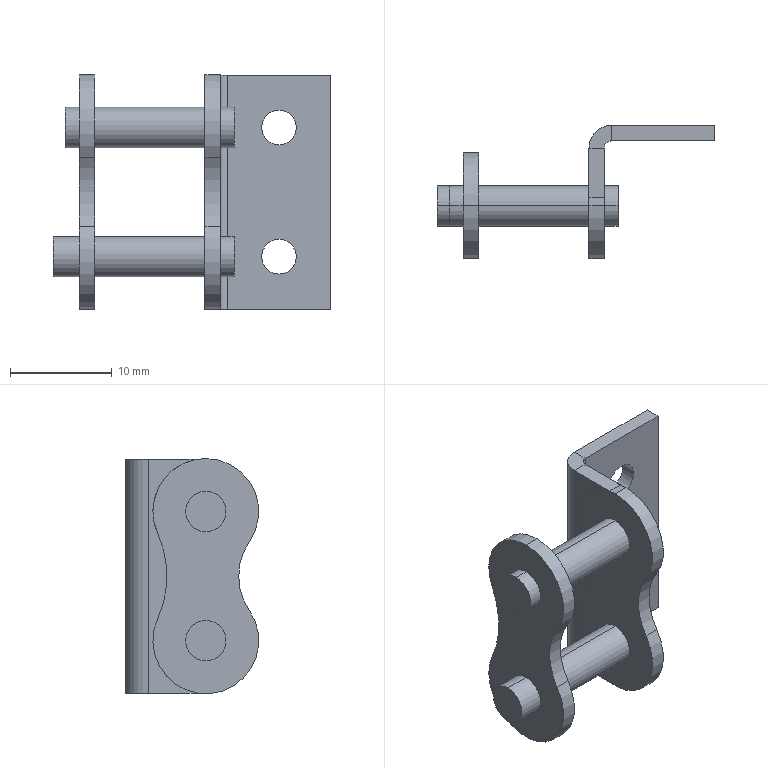Part | SolidWorks | features MoveFace 9, 3DProfileFeature 1, BaseBody 1, EdgeFlange 1, FlatPattern 1, HoleWzd 1, SMBaseFlange 1, SheetMetal 1 | 2 solids | 50 faces | box 27.296 x 13.105 x 23.11 mm | volume 1387 mm3 | cylinder 31 | plane 19 | commonest cylinder face diameters 3.98 x12 10.41 x8 3.4 x4 20 x3 12 x2 1.473 x1
STEP:
#1=CARTESIAN_POINT('',(12.2,6.4,-11.));
#2=VERTEX_POINT('',#1);
#3=CARTESIAN_POINT('',(12.2,6.4,-14.4));
#4=VERTEX_POINT('',#3);
#5=CARTESIAN_POINT('',(12.2,6.4,-12.7));
#6=DIRECTION('',(0.,-1.,0.));
#7=DIRECTION('',(1.,0.,0.));
#8=AXIS2_PLACEMENT_3D('',#5,#6,#7);
#9=CIRCLE('',#8,1.7);
#10=EDGE_CURVE('',#2,#4,#9,.T.);
#11=ORIENTED_EDGE('',*,*,#10,.T.);
#12=CARTESIAN_POINT('',(12.2,7.9,-14.4));
#13=VERTEX_POINT('',#12);
#14=CARTESIAN_POINT('',(12.2,7.9,-14.4));
#15=DIRECTION('',(0.,1.,0.));
#16=VECTOR('',#15,1000.);
#17=LINE('',#14,#16);
#18=EDGE_CURVE('',#4,#13,#17,.T.);
#19=ORIENTED_EDGE('',*,*,#18,.T.);
#20=CARTESIAN_POINT('',(12.2,7.9,-11.));
#21=VERTEX_POINT('',#20);
#22=CARTESIAN_POINT('',(12.2,7.9,-12.7));
#23=DIRECTION('',(0.,1.,0.));
#24=DIRECTION('',(0.,0.,1.));
#25=AXIS2_PLACEMENT_3D('',#22,#23,#24);
#26=CIRCLE('',#25,1.7);
#27=EDGE_CURVE('',#13,#21,#26,.T.);
#28=ORIENTED_EDGE('',*,*,#27,.T.);
#29=CARTESIAN_POINT('',(12.2,7.9,-11.));
#30=DIRECTION('',(0.,1.,0.));
#31=VECTOR('',#30,1000.);
#32=LINE('',#29,#31);
#33=EDGE_CURVE('',#2,#21,#32,.T.);
#34=ORIENTED_EDGE('',*,*,#33,.F.);
#35=EDGE_LOOP('',(#11,#19,#28,#34));
#36=FACE_OUTER_BOUND('',#35,.T.);
#37=CARTESIAN_POINT('',(12.2,7.9,-12.7));
#38=DIRECTION('',(0.,1.,0.));
#39=DIRECTION('',(0.,0.,1.));
#40=AXIS2_PLACEMENT_3D('',#37,#38,#39);
#41=CYLINDRICAL_SURFACE('',#40,1.7);
#42=ADVANCED_FACE('',(#36),#41,.F.);
#43=CARTESIAN_POINT('',(12.2,6.4,1.7));
#44=VERTEX_POINT('',#43);
#45=CARTESIAN_POINT('',(12.2,6.4,-1.7));
#46=VERTEX_POINT('',#45);
#47=CARTESIAN_POINT('',(12.2,6.4,0.));
#48=DIRECTION('',(0.,-1.,0.));
#49=DIRECTION('',(1.,0.,0.));
#50=AXIS2_PLACEMENT_3D('',#47,#48,#49);
#51=CIRCLE('',#50,1.7);
#52=EDGE_CURVE('',#44,#46,#51,.T.);
#53=ORIENTED_EDGE('',*,*,#52,.T.);
#54=CARTESIAN_POINT('',(12.2,7.9,-1.7));
#55=VERTEX_POINT('',#54);
#56=CARTESIAN_POINT('',(12.2,7.9,-1.7));
#57=DIRECTION('',(0.,1.,0.));
#58=VECTOR('',#57,1000.);
#59=LINE('',#56,#58);
#60=EDGE_CURVE('',#46,#55,#59,.T.);
#61=ORIENTED_EDGE('',*,*,#60,.T.);
#62=CARTESIAN_POINT('',(12.2,7.9,1.7));
#63=VERTEX_POINT('',#62);
#64=CARTESIAN_POINT('',(12.2,7.9,0.));
#65=DIRECTION('',(0.,1.,0.));
#66=DIRECTION('',(0.,0.,1.));
#67=AXIS2_PLACEMENT_3D('',#64,#65,#66);
#68=CIRCLE('',#67,1.7);
#69=EDGE_CURVE('',#55,#63,#68,.T.);
#70=ORIENTED_EDGE('',*,*,#69,.T.);
#71=CARTESIAN_POINT('',(12.2,7.9,1.7));
#72=DIRECTION('',(0.,1.,0.));
#73=VECTOR('',#72,1000.);
#74=LINE('',#71,#73);
#75=EDGE_CURVE('',#44,#63,#74,.T.);
#76=ORIENTED_EDGE('',*,*,#75,.F.);
#77=EDGE_LOOP('',(#53,#61,#70,#76));
#78=FACE_OUTER_BOUND('',#77,.T.);
#79=CARTESIAN_POINT('',(12.2,7.9,0.));
#80=DIRECTION('',(0.,1.,0.));
#81=DIRECTION('',(0.,0.,1.));
#82=AXIS2_PLACEMENT_3D('',#79,#80,#81);
#83=CYLINDRICAL_SURFACE('',#82,1.7);
#84=ADVANCED_FACE('',(#78),#83,.F.);
#85=CARTESIAN_POINT('',(6.425,0.7547,5.15));
#86=VERTEX_POINT('',#85);
#87=CARTESIAN_POINT('',(6.425,5.663,5.15));
#88=VERTEX_POINT('',#87);
#89=CARTESIAN_POINT('',(6.425,0.7547,5.15));
#90=DIRECTION('',(0.,1.,0.));
#91=VECTOR('',#90,1000.);
#92=LINE('',#89,#91);
#93=EDGE_CURVE('',#86,#88,#92,.T.);
#94=ORIENTED_EDGE('',*,*,#93,.T.);
#95=CARTESIAN_POINT('',(4.925,5.663,5.15));
#96=VERTEX_POINT('',#95);
#97=CARTESIAN_POINT('',(6.425,5.663,5.15));
#98=DIRECTION('',(-1.,0.,0.));
#99=VECTOR('',#98,1000.);
#100=LINE('',#97,#99);
#101=EDGE_CURVE('',#88,#96,#100,.T.);
#102=ORIENTED_EDGE('',*,*,#101,.T.);
#103=CARTESIAN_POINT('',(4.925,0.7547,5.15));
#104=VERTEX_POINT('',#103);
#105=CARTESIAN_POINT('',(4.925,0.7547,5.15));
#106=DIRECTION('',(0.,1.,0.));
#107=VECTOR('',#106,1000.);
#108=LINE('',#105,#107);
#109=EDGE_CURVE('',#104,#96,#108,.T.);
#110=ORIENTED_EDGE('',*,*,#109,.F.);
#111=CARTESIAN_POINT('',(7.425,0.7547,5.15));
#112=DIRECTION('',(-1.,0.,0.));
#113=VECTOR('',#112,1000.);
#114=LINE('',#111,#113);
#115=EDGE_CURVE('',#86,#104,#114,.T.);
#116=ORIENTED_EDGE('',*,*,#115,.F.);
#117=EDGE_LOOP('',(#94,#102,#110,#116));
#118=FACE_OUTER_BOUND('',#117,.T.);
#119=CARTESIAN_POINT('',(7.425,0.7547,5.15));
#120=DIRECTION('',(0.,0.,1.));
#121=DIRECTION('',(1.,0.,0.));
#122=AXIS2_PLACEMENT_3D('',#119,#120,#121);
#123=PLANE('',#122);
#124=ADVANCED_FACE('',(#118),#123,.T.);
#125=CARTESIAN_POINT('',(6.425,5.663,-17.85));
#126=VERTEX_POINT('',#125);
#127=CARTESIAN_POINT('',(6.425,5.663,5.15));
#128=DIRECTION('',(0.,0.,-1.));
#129=VECTOR('',#128,1000.);
#130=LINE('',#127,#129);
#131=EDGE_CURVE('',#88,#126,#130,.T.);
#132=ORIENTED_EDGE('',*,*,#131,.F.);
#133=ORIENTED_EDGE('',*,*,#93,.F.);
#134=CARTESIAN_POINT('',(6.425,4.729,-2.174));
#135=VERTEX_POINT('',#134);
#136=CARTESIAN_POINT('',(6.425,0.,0.));
#137=DIRECTION('',(1.,0.,0.));
#138=DIRECTION('',(0.,0.,1.));
#139=AXIS2_PLACEMENT_3D('',#136,#137,#138);
#140=CIRCLE('',#139,5.205);
#141=EDGE_CURVE('',#135,#86,#140,.T.);
#142=ORIENTED_EDGE('',*,*,#141,.F.);
#143=CARTESIAN_POINT('',(6.425,4.729,-10.526));
#144=VERTEX_POINT('',#143);
#145=CARTESIAN_POINT('',(6.425,13.816,-6.35));
#146=DIRECTION('',(-1.,0.,0.));
#147=DIRECTION('',(0.,0.,1.));
#148=AXIS2_PLACEMENT_3D('',#145,#146,#147);
#149=CIRCLE('',#148,10.);
#150=EDGE_CURVE('',#144,#135,#149,.T.);
#151=ORIENTED_EDGE('',*,*,#150,.F.);
#152=CARTESIAN_POINT('',(6.425,0.7547,-17.85));
#153=VERTEX_POINT('',#152);
#154=CARTESIAN_POINT('',(6.425,0.,-12.7));
#155=DIRECTION('',(1.,0.,0.));
#156=DIRECTION('',(0.,0.,1.));
#157=AXIS2_PLACEMENT_3D('',#154,#155,#156);
#158=CIRCLE('',#157,5.205);
#159=EDGE_CURVE('',#153,#144,#158,.T.);
#160=ORIENTED_EDGE('',*,*,#159,.F.);
#161=CARTESIAN_POINT('',(6.425,7.9,-17.85));
#162=DIRECTION('',(0.,-1.,0.));
#163=VECTOR('',#162,1000.);
#164=LINE('',#161,#163);
#165=EDGE_CURVE('',#126,#153,#164,.T.);
#166=ORIENTED_EDGE('',*,*,#165,.F.);
#167=EDGE_LOOP('',(#132,#133,#142,#151,#160,#166));
#168=FACE_OUTER_BOUND('',#167,.T.);
#169=CARTESIAN_POINT('',(6.425,0.,0.));
#170=DIRECTION('',(-1.,0.,0.));
#171=DIRECTION('',(0.,0.,1.));
#172=AXIS2_PLACEMENT_3D('',#169,#170,#171);
#173=PLANE('',#172);
#174=ADVANCED_FACE('',(#168),#173,.F.);
#175=ORIENTED_EDGE('',*,*,#109,.T.);
#176=CARTESIAN_POINT('',(4.925,5.663,-17.85));
#177=VERTEX_POINT('',#176);
#178=CARTESIAN_POINT('',(4.925,5.663,5.15));
#179=DIRECTION('',(0.,0.,-1.));
#180=VECTOR('',#179,1000.);
#181=LINE('',#178,#180);
#182=EDGE_CURVE('',#96,#177,#181,.T.);
#183=ORIENTED_EDGE('',*,*,#182,.T.);
#184=CARTESIAN_POINT('',(4.925,0.7547,-17.85));
#185=VERTEX_POINT('',#184);
#186=CARTESIAN_POINT('',(4.925,7.9,-17.85));
#187=DIRECTION('',(0.,-1.,0.));
#188=VECTOR('',#187,1000.);
#189=LINE('',#186,#188);
#190=EDGE_CURVE('',#177,#185,#189,.T.);
#191=ORIENTED_EDGE('',*,*,#190,.T.);
#192=CARTESIAN_POINT('',(4.925,4.729,-10.526));
#193=VERTEX_POINT('',#192);
#194=CARTESIAN_POINT('',(4.925,0.,-12.7));
#195=DIRECTION('',(1.,0.,0.));
#196=DIRECTION('',(0.,0.,1.));
#197=AXIS2_PLACEMENT_3D('',#194,#195,#196);
#198=CIRCLE('',#197,5.205);
#199=EDGE_CURVE('',#185,#193,#198,.T.);
#200=ORIENTED_EDGE('',*,*,#199,.T.);
#201=CARTESIAN_POINT('',(4.925,4.729,-2.174));
#202=VERTEX_POINT('',#201);
#203=CARTESIAN_POINT('',(4.925,13.816,-6.35));
#204=DIRECTION('',(-1.,0.,0.));
#205=DIRECTION('',(0.,0.,1.));
#206=AXIS2_PLACEMENT_3D('',#203,#204,#205);
#207=CIRCLE('',#206,10.);
#208=EDGE_CURVE('',#193,#202,#207,.T.);
#209=ORIENTED_EDGE('',*,*,#208,.T.);
#210=CARTESIAN_POINT('',(4.925,0.,0.));
#211=DIRECTION('',(1.,0.,0.));
#212=DIRECTION('',(0.,0.,1.));
#213=AXIS2_PLACEMENT_3D('',#210,#211,#212);
#214=CIRCLE('',#213,5.205);
#215=EDGE_CURVE('',#202,#104,#214,.T.);
#216=ORIENTED_EDGE('',*,*,#215,.T.);
#217=EDGE_LOOP('',(#175,#183,#191,#200,#209,#216));
#218=FACE_OUTER_BOUND('',#217,.T.);
#219=CARTESIAN_POINT('',(4.925,0.,0.));
#220=DIRECTION('',(-1.,0.,0.));
#221=DIRECTION('',(0.,0.,1.));
#222=AXIS2_PLACEMENT_3D('',#219,#220,#221);
#223=PLANE('',#222);
#224=ADVANCED_FACE('',(#218),#223,.T.);
#225=ORIENTED_EDGE('',*,*,#215,.F.);
#226=CARTESIAN_POINT('',(7.425,4.729,-2.174));
#227=DIRECTION('',(-1.,0.,0.));
#228=VECTOR('',#227,1000.);
#229=LINE('',#226,#228);
#230=EDGE_CURVE('',#135,#202,#229,.T.);
#231=ORIENTED_EDGE('',*,*,#230,.F.);
#232=ORIENTED_EDGE('',*,*,#141,.T.);
#233=ORIENTED_EDGE('',*,*,#115,.T.);
#234=EDGE_LOOP('',(#225,#231,#232,#233));
#235=FACE_OUTER_BOUND('',#234,.T.);
#236=CARTESIAN_POINT('',(7.425,0.,0.));
#237=DIRECTION('',(-1.,0.,0.));
#238=DIRECTION('',(0.,0.,1.));
#239=AXIS2_PLACEMENT_3D('',#236,#237,#238);
#240=CYLINDRICAL_SURFACE('',#239,5.205);
#241=ADVANCED_FACE('',(#235),#240,.F.);
#242=ORIENTED_EDGE('',*,*,#208,.F.);
#243=CARTESIAN_POINT('',(7.425,4.729,-10.526));
#244=DIRECTION('',(-1.,0.,0.));
#245=VECTOR('',#244,1000.);
#246=LINE('',#243,#245);
#247=EDGE_CURVE('',#144,#193,#246,.T.);
#248=ORIENTED_EDGE('',*,*,#247,.F.);
#249=ORIENTED_EDGE('',*,*,#150,.T.);
#250=ORIENTED_EDGE('',*,*,#230,.T.);
#251=EDGE_LOOP('',(#242,#248,#249,#250));
#252=FACE_OUTER_BOUND('',#251,.T.);
#253=CARTESIAN_POINT('',(7.425,13.816,-6.35));
#254=DIRECTION('',(-1.,0.,0.));
#255=DIRECTION('',(0.,0.,1.));
#256=AXIS2_PLACEMENT_3D('',#253,#254,#255);
#257=CYLINDRICAL_SURFACE('',#256,10.);
#258=ADVANCED_FACE('',(#252),#257,.T.);
#259=ORIENTED_EDGE('',*,*,#199,.F.);
#260=CARTESIAN_POINT('',(7.425,0.7547,-17.85));
#261=DIRECTION('',(-1.,0.,0.));
#262=VECTOR('',#261,1000.);
#263=LINE('',#260,#262);
#264=EDGE_CURVE('',#153,#185,#263,.T.);
#265=ORIENTED_EDGE('',*,*,#264,.F.);
#266=ORIENTED_EDGE('',*,*,#159,.T.);
#267=ORIENTED_EDGE('',*,*,#247,.T.);
#268=EDGE_LOOP('',(#259,#265,#266,#267));
#269=FACE_OUTER_BOUND('',#268,.T.);
#270=CARTESIAN_POINT('',(7.425,0.,-12.7));
#271=DIRECTION('',(-1.,0.,0.));
#272=DIRECTION('',(0.,0.,1.));
#273=AXIS2_PLACEMENT_3D('',#270,#271,#272);
#274=CYLINDRICAL_SURFACE('',#273,5.205);
#275=ADVANCED_FACE('',(#269),#274,.F.);
#276=CARTESIAN_POINT('',(6.425,5.663,-17.85));
#277=DIRECTION('',(-1.,0.,0.));
#278=VECTOR('',#277,1000.);
#279=LINE('',#276,#278);
#280=EDGE_CURVE('',#126,#177,#279,.T.);
#281=ORIENTED_EDGE('',*,*,#280,.F.);
#282=ORIENTED_EDGE('',*,*,#165,.T.);
#283=ORIENTED_EDGE('',*,*,#264,.T.);
#284=ORIENTED_EDGE('',*,*,#190,.F.);
#285=EDGE_LOOP('',(#281,#282,#283,#284));
#286=FACE_OUTER_BOUND('',#285,.T.);
#287=CARTESIAN_POINT('',(7.425,7.9,-17.85));
#288=DIRECTION('',(0.,0.,-1.));
#289=DIRECTION('',(-1.,0.,0.));
#290=AXIS2_PLACEMENT_3D('',#287,#288,#289);
#291=PLANE('',#290);
#292=ADVANCED_FACE('',(#286),#291,.T.);
#293=CARTESIAN_POINT('',(7.162,6.4,-17.85));
#294=VERTEX_POINT('',#293);
#295=CARTESIAN_POINT('',(7.162,7.9,-17.85));
#296=VERTEX_POINT('',#295);
#297=CARTESIAN_POINT('',(7.162,7.9,-17.85));
#298=DIRECTION('',(0.,1.,0.));
#299=VECTOR('',#298,1000.);
#300=LINE('',#297,#299);
#301=EDGE_CURVE('',#294,#296,#300,.T.);
#302=ORIENTED_EDGE('',*,*,#301,.F.);
#303=CARTESIAN_POINT('',(7.162,5.663,-17.85));
#304=DIRECTION('',(0.,0.,-1.));
#305=DIRECTION('',(1.,0.,0.));
#306=AXIS2_PLACEMENT_3D('',#303,#304,#305);
#307=CIRCLE('',#306,0.7366);
#308=EDGE_CURVE('',#126,#294,#307,.T.);
#309=ORIENTED_EDGE('',*,*,#308,.F.);
#310=ORIENTED_EDGE('',*,*,#280,.T.);
#311=CARTESIAN_POINT('',(7.162,5.663,-17.85));
#312=DIRECTION('',(0.,0.,-1.));
#313=DIRECTION('',(1.,0.,0.));
#314=AXIS2_PLACEMENT_3D('',#311,#312,#313);
#315=CIRCLE('',#314,2.237);
#316=EDGE_CURVE('',#177,#296,#315,.T.);
#317=ORIENTED_EDGE('',*,*,#316,.T.);
#318=EDGE_LOOP('',(#302,#309,#310,#317));
#319=FACE_OUTER_BOUND('',#318,.T.);
#320=CARTESIAN_POINT('',(7.162,5.663,-17.85));
#321=DIRECTION('',(0.,0.,-1.));
#322=DIRECTION('',(-1.,0.,0.));
#323=AXIS2_PLACEMENT_3D('',#320,#321,#322);
#324=PLANE('',#323);
#325=ADVANCED_FACE('',(#319),#324,.T.);
#326=CARTESIAN_POINT('',(7.162,6.4,5.15));
#327=VERTEX_POINT('',#326);
#328=CARTESIAN_POINT('',(7.162,5.663,5.15));
#329=DIRECTION('',(0.,0.,1.));
#330=DIRECTION('',(1.,0.,0.));
#331=AXIS2_PLACEMENT_3D('',#328,#329,#330);
#332=CIRCLE('',#331,0.7366);
#333=EDGE_CURVE('',#327,#88,#332,.T.);
#334=ORIENTED_EDGE('',*,*,#333,.F.);
#335=CARTESIAN_POINT('',(7.162,7.9,5.15));
#336=VERTEX_POINT('',#335);
#337=CARTESIAN_POINT('',(7.162,6.4,5.15));
#338=DIRECTION('',(0.,1.,0.));
#339=VECTOR('',#338,1000.);
#340=LINE('',#337,#339);
#341=EDGE_CURVE('',#327,#336,#340,.T.);
#342=ORIENTED_EDGE('',*,*,#341,.T.);
#343=CARTESIAN_POINT('',(7.162,5.663,5.15));
#344=DIRECTION('',(0.,0.,1.));
#345=DIRECTION('',(1.,0.,0.));
#346=AXIS2_PLACEMENT_3D('',#343,#344,#345);
#347=CIRCLE('',#346,2.237);
#348=EDGE_CURVE('',#336,#96,#347,.T.);
#349=ORIENTED_EDGE('',*,*,#348,.T.);
#350=ORIENTED_EDGE('',*,*,#101,.F.);
#351=EDGE_LOOP('',(#334,#342,#349,#350));
#352=FACE_OUTER_BOUND('',#351,.T.);
#353=CARTESIAN_POINT('',(7.162,5.663,5.15));
#354=DIRECTION('',(0.,0.,-1.));
#355=DIRECTION('',(-1.,0.,0.));
#356=AXIS2_PLACEMENT_3D('',#353,#354,#355);
#357=PLANE('',#356);
#358=ADVANCED_FACE('',(#352),#357,.F.);
#359=ORIENTED_EDGE('',*,*,#182,.F.);
#360=ORIENTED_EDGE('',*,*,#348,.F.);
#361=CARTESIAN_POINT('',(7.162,7.9,-17.85));
#362=DIRECTION('',(0.,0.,-1.));
#363=VECTOR('',#362,1000.);
#364=LINE('',#361,#363);
#365=EDGE_CURVE('',#336,#296,#364,.T.);
#366=ORIENTED_EDGE('',*,*,#365,.T.);
#367=ORIENTED_EDGE('',*,*,#316,.F.);
#368=EDGE_LOOP('',(#359,#360,#366,#367));
#369=FACE_OUTER_BOUND('',#368,.T.);
#370=CARTESIAN_POINT('',(7.162,5.663,5.15));
#371=DIRECTION('',(0.,0.,1.));
#372=DIRECTION('',(0.,1.,0.));
#373=AXIS2_PLACEMENT_3D('',#370,#371,#372);
#374=CYLINDRICAL_SURFACE('',#373,2.237);
#375=ADVANCED_FACE('',(#369),#374,.T.);
#376=ORIENTED_EDGE('',*,*,#131,.T.);
#377=ORIENTED_EDGE('',*,*,#308,.T.);
#378=CARTESIAN_POINT('',(7.162,6.4,-17.85));
#379=DIRECTION('',(0.,0.,1.));
#380=VECTOR('',#379,1000.);
#381=LINE('',#378,#380);
#382=EDGE_CURVE('',#294,#327,#381,.T.);
#383=ORIENTED_EDGE('',*,*,#382,.T.);
#384=ORIENTED_EDGE('',*,*,#333,.T.);
#385=EDGE_LOOP('',(#376,#377,#383,#384));
#386=FACE_OUTER_BOUND('',#385,.T.);
#387=CARTESIAN_POINT('',(7.162,5.663,5.15));
#388=DIRECTION('',(0.,0.,1.));
#389=DIRECTION('',(0.,1.,0.));
#390=AXIS2_PLACEMENT_3D('',#387,#388,#389);
#391=CYLINDRICAL_SURFACE('',#390,0.7366);
#392=ADVANCED_FACE('',(#386),#391,.F.);
#393=ORIENTED_EDGE('',*,*,#341,.F.);
#394=CARTESIAN_POINT('',(17.3,6.4,5.15));
#395=VERTEX_POINT('',#394);
#396=CARTESIAN_POINT('',(17.3,6.4,5.15));
#397=DIRECTION('',(1.,0.,0.));
#398=VECTOR('',#397,1000.);
#399=LINE('',#396,#398);
#400=EDGE_CURVE('',#327,#395,#399,.T.);
#401=ORIENTED_EDGE('',*,*,#400,.T.);
#402=CARTESIAN_POINT('',(17.3,7.9,5.15));
#403=VERTEX_POINT('',#402);
#404=CARTESIAN_POINT('',(17.3,7.9,5.15));
#405=DIRECTION('',(0.,-1.,0.));
#406=VECTOR('',#405,1000.);
#407=LINE('',#404,#406);
#408=EDGE_CURVE('',#403,#395,#407,.T.);
#409=ORIENTED_EDGE('',*,*,#408,.F.);
#410=CARTESIAN_POINT('',(0.,7.9,5.15));
#411=DIRECTION('',(1.,0.,0.));
#412=VECTOR('',#411,1000.);
#413=LINE('',#410,#412);
#414=EDGE_CURVE('',#336,#403,#413,.T.);
#415=ORIENTED_EDGE('',*,*,#414,.F.);
#416=EDGE_LOOP('',(#393,#401,#409,#415));
#417=FACE_OUTER_BOUND('',#416,.T.);
#418=CARTESIAN_POINT('',(17.3,7.9,5.15));
#419=DIRECTION('',(0.,0.,-1.));
#420=DIRECTION('',(-1.,0.,0.));
#421=AXIS2_PLACEMENT_3D('',#418,#419,#420);
#422=PLANE('',#421);
#423=ADVANCED_FACE('',(#417),#422,.F.);
#424=ORIENTED_EDGE('',*,*,#301,.T.);
#425=CARTESIAN_POINT('',(17.3,7.9,-17.85));
#426=VERTEX_POINT('',#425);
#427=CARTESIAN_POINT('',(0.,7.9,-17.85));
#428=DIRECTION('',(-1.,0.,0.));
#429=VECTOR('',#428,1000.);
#430=LINE('',#427,#429);
#431=EDGE_CURVE('',#426,#296,#430,.T.);
#432=ORIENTED_EDGE('',*,*,#431,.F.);
#433=CARTESIAN_POINT('',(17.3,6.4,-17.85));
#434=VERTEX_POINT('',#433);
#435=CARTESIAN_POINT('',(17.3,7.9,-17.85));
#436=DIRECTION('',(0.,-1.,0.));
#437=VECTOR('',#436,1000.);
#438=LINE('',#435,#437);
#439=EDGE_CURVE('',#426,#434,#438,.T.);
#440=ORIENTED_EDGE('',*,*,#439,.T.);
#441=CARTESIAN_POINT('',(6.425,6.4,-17.85));
#442=DIRECTION('',(-1.,0.,0.));
#443=VECTOR('',#442,1000.);
#444=LINE('',#441,#443);
#445=EDGE_CURVE('',#434,#294,#444,.T.);
#446=ORIENTED_EDGE('',*,*,#445,.T.);
#447=EDGE_LOOP('',(#424,#432,#440,#446));
#448=FACE_OUTER_BOUND('',#447,.T.);
#449=CARTESIAN_POINT('',(6.425,7.9,-17.85));
#450=DIRECTION('',(0.,0.,1.));
#451=DIRECTION('',(1.,0.,0.));
#452=AXIS2_PLACEMENT_3D('',#449,#450,#451);
#453=PLANE('',#452);
#454=ADVANCED_FACE('',(#448),#453,.F.);
#455=CARTESIAN_POINT('',(12.2,7.9,-12.7));
#456=DIRECTION('',(0.,1.,0.));
#457=DIRECTION('',(0.,0.,1.));
#458=AXIS2_PLACEMENT_3D('',#455,#456,#457);
#459=CIRCLE('',#458,1.7);
#460=EDGE_CURVE('',#21,#13,#459,.T.);
#461=ORIENTED_EDGE('',*,*,#460,.F.);
#462=ORIENTED_EDGE('',*,*,#27,.F.);
#463=EDGE_LOOP('',(#461,#462));
#464=FACE_BOUND('',#463,.T.);
#465=CARTESIAN_POINT('',(12.2,7.9,0.));
#466=DIRECTION('',(0.,1.,0.));
#467=DIRECTION('',(0.,0.,1.));
#468=AXIS2_PLACEMENT_3D('',#465,#466,#467);
#469=CIRCLE('',#468,1.7);
#470=EDGE_CURVE('',#63,#55,#469,.T.);
#471=ORIENTED_EDGE('',*,*,#470,.F.);
#472=ORIENTED_EDGE('',*,*,#69,.F.);
#473=EDGE_LOOP('',(#471,#472));
#474=FACE_BOUND('',#473,.T.);
#475=ORIENTED_EDGE('',*,*,#365,.F.);
#476=ORIENTED_EDGE('',*,*,#414,.T.);
#477=CARTESIAN_POINT('',(17.3,7.9,0.));
#478=DIRECTION('',(0.,0.,-1.));
#479=VECTOR('',#478,1000.);
#480=LINE('',#477,#479);
#481=EDGE_CURVE('',#403,#426,#480,.T.);
#482=ORIENTED_EDGE('',*,*,#481,.T.);
#483=ORIENTED_EDGE('',*,*,#431,.T.);
#484=EDGE_LOOP('',(#475,#476,#482,#483));
#485=FACE_OUTER_BOUND('',#484,.T.);
#486=CARTESIAN_POINT('',(0.,7.9,0.));
#487=DIRECTION('',(0.,-1.,0.));
#488=DIRECTION('',(1.,0.,0.));
#489=AXIS2_PLACEMENT_3D('',#486,#487,#488);
#490=PLANE('',#489);
#491=ADVANCED_FACE('',(#464,#474,#485),#490,.F.);
#492=ORIENTED_EDGE('',*,*,#10,.F.);
#493=CARTESIAN_POINT('',(12.2,6.4,-12.7));
#494=DIRECTION('',(0.,-1.,0.));
#495=DIRECTION('',(1.,0.,0.));
#496=AXIS2_PLACEMENT_3D('',#493,#494,#495);
#497=CIRCLE('',#496,1.7);
#498=EDGE_CURVE('',#4,#2,#497,.T.);
#499=ORIENTED_EDGE('',*,*,#498,.F.);
#500=EDGE_LOOP('',(#492,#499));
#501=FACE_BOUND('',#500,.T.);
#502=ORIENTED_EDGE('',*,*,#52,.F.);
#503=CARTESIAN_POINT('',(12.2,6.4,0.));
#504=DIRECTION('',(0.,-1.,0.));
#505=DIRECTION('',(1.,0.,0.));
#506=AXIS2_PLACEMENT_3D('',#503,#504,#505);
#507=CIRCLE('',#506,1.7);
#508=EDGE_CURVE('',#46,#44,#507,.T.);
#509=ORIENTED_EDGE('',*,*,#508,.F.);
#510=EDGE_LOOP('',(#502,#509));
#511=FACE_BOUND('',#510,.T.);
#512=ORIENTED_EDGE('',*,*,#400,.F.);
#513=ORIENTED_EDGE('',*,*,#382,.F.);
#514=ORIENTED_EDGE('',*,*,#445,.F.);
#515=CARTESIAN_POINT('',(17.3,6.4,-17.85));
#516=DIRECTION('',(0.,0.,-1.));
#517=VECTOR('',#516,1000.);
#518=LINE('',#515,#517);
#519=EDGE_CURVE('',#395,#434,#518,.T.);
#520=ORIENTED_EDGE('',*,*,#519,.F.);
#521=EDGE_LOOP('',(#512,#513,#514,#520));
#522=FACE_OUTER_BOUND('',#521,.T.);
#523=CARTESIAN_POINT('',(0.,6.4,0.));
#524=DIRECTION('',(0.,-1.,0.));
#525=DIRECTION('',(1.,0.,0.));
#526=AXIS2_PLACEMENT_3D('',#523,#524,#525);
#527=PLANE('',#526);
#528=ADVANCED_FACE('',(#501,#511,#522),#527,.T.);
#529=ORIENTED_EDGE('',*,*,#519,.T.);
#530=ORIENTED_EDGE('',*,*,#439,.F.);
#531=ORIENTED_EDGE('',*,*,#481,.F.);
#532=ORIENTED_EDGE('',*,*,#408,.T.);
#533=EDGE_LOOP('',(#529,#530,#531,#532));
#534=FACE_OUTER_BOUND('',#533,.T.);
#535=CARTESIAN_POINT('',(17.3,7.9,-17.85));
#536=DIRECTION('',(-1.,0.,0.));
#537=DIRECTION('',(0.,-1.,0.));
#538=AXIS2_PLACEMENT_3D('',#535,#536,#537);
#539=PLANE('',#538);
#540=ADVANCED_FACE('',(#534),#539,.F.);
#541=ORIENTED_EDGE('',*,*,#60,.F.);
#542=ORIENTED_EDGE('',*,*,#508,.T.);
#543=ORIENTED_EDGE('',*,*,#75,.T.);
#544=ORIENTED_EDGE('',*,*,#470,.T.);
#545=EDGE_LOOP('',(#541,#542,#543,#544));
#546=FACE_OUTER_BOUND('',#545,.T.);
#547=CARTESIAN_POINT('',(12.2,7.9,0.));
#548=DIRECTION('',(0.,1.,0.));
#549=DIRECTION('',(0.,0.,1.));
#550=AXIS2_PLACEMENT_3D('',#547,#548,#549);
#551=CYLINDRICAL_SURFACE('',#550,1.7);
#552=ADVANCED_FACE('',(#546),#551,.F.);
#553=ORIENTED_EDGE('',*,*,#18,.F.);
#554=ORIENTED_EDGE('',*,*,#498,.T.);
#555=ORIENTED_EDGE('',*,*,#33,.T.);
#556=ORIENTED_EDGE('',*,*,#460,.T.);
#557=EDGE_LOOP('',(#553,#554,#555,#556));
#558=FACE_OUTER_BOUND('',#557,.T.);
#559=CARTESIAN_POINT('',(12.2,7.9,-12.7));
#560=DIRECTION('',(0.,1.,0.));
#561=DIRECTION('',(0.,0.,1.));
#562=AXIS2_PLACEMENT_3D('',#559,#560,#561);
#563=CYLINDRICAL_SURFACE('',#562,1.7);
#564=ADVANCED_FACE('',(#558),#563,.F.);
#565=CLOSED_SHELL('',(#42,#84,#124,#174,#224,#241,#258,#275,#292,#325,#358,#375,#392,#423,#454,#491,#528,#540,#552,#564));
#566=MANIFOLD_SOLID_BREP('',#565);
#567=CARTESIAN_POINT('',(-9.996,0.,-10.71));
#568=VERTEX_POINT('',#567);
#569=CARTESIAN_POINT('',(-9.996,0.,-14.69));
#570=VERTEX_POINT('',#569);
#571=CARTESIAN_POINT('',(-9.996,0.,-12.7));
#572=DIRECTION('',(1.,0.,0.));
#573=DIRECTION('',(0.,0.,-1.));
#574=AXIS2_PLACEMENT_3D('',#571,#572,#573);
#575=CIRCLE('',#574,1.99);
#576=EDGE_CURVE('',#568,#570,#575,.T.);
#577=ORIENTED_EDGE('',*,*,#576,.T.);
#578=CARTESIAN_POINT('',(-7.425,0.,-14.69));
#579=VERTEX_POINT('',#578);
#580=CARTESIAN_POINT('',(8.13,0.,-14.69));
#581=DIRECTION('',(1.,0.,0.));
#582=VECTOR('',#581,1000.);
#583=LINE('',#580,#582);
#584=EDGE_CURVE('',#570,#579,#583,.T.);
#585=ORIENTED_EDGE('',*,*,#584,.T.);
#586=CARTESIAN_POINT('',(-7.425,0.,-10.71));
#587=VERTEX_POINT('',#586);
#588=CARTESIAN_POINT('',(-7.425,0.,-12.7));
#589=DIRECTION('',(-1.,0.,0.));
#590=DIRECTION('',(0.,0.,-1.));
#591=AXIS2_PLACEMENT_3D('',#588,#589,#590);
#592=CIRCLE('',#591,1.99);
#593=EDGE_CURVE('',#579,#587,#592,.T.);
#594=ORIENTED_EDGE('',*,*,#593,.T.);
#595=CARTESIAN_POINT('',(8.13,0.,-10.71));
#596=DIRECTION('',(1.,0.,0.));
#597=VECTOR('',#596,1000.);
#598=LINE('',#595,#597);
#599=EDGE_CURVE('',#568,#587,#598,.T.);
#600=ORIENTED_EDGE('',*,*,#599,.F.);
#601=EDGE_LOOP('',(#577,#585,#594,#600));
#602=FACE_OUTER_BOUND('',#601,.T.);
#603=CARTESIAN_POINT('',(8.13,0.,-12.7));
#604=DIRECTION('',(1.,0.,0.));
#605=DIRECTION('',(0.,0.,1.));
#606=AXIS2_PLACEMENT_3D('',#603,#604,#605);
#607=CYLINDRICAL_SURFACE('',#606,1.99);
#608=ADVANCED_FACE('',(#602),#607,.T.);
#609=CARTESIAN_POINT('',(-7.425,4.729,-2.174));
#610=VERTEX_POINT('',#609);
#611=CARTESIAN_POINT('',(-7.425,0.,5.205));
#612=VERTEX_POINT('',#611);
#613=CARTESIAN_POINT('',(-7.425,0.,0.));
#614=DIRECTION('',(1.,0.,0.));
#615=DIRECTION('',(0.,0.,-1.));
#616=AXIS2_PLACEMENT_3D('',#613,#614,#615);
#617=CIRCLE('',#616,5.205);
#618=EDGE_CURVE('',#610,#612,#617,.T.);
#619=ORIENTED_EDGE('',*,*,#618,.T.);
#620=CARTESIAN_POINT('',(-5.925,0.,5.205));
#621=VERTEX_POINT('',#620);
#622=CARTESIAN_POINT('',(7.925,0.,5.205));
#623=DIRECTION('',(1.,0.,0.));
#624=VECTOR('',#623,1000.);
#625=LINE('',#622,#624);
#626=EDGE_CURVE('',#612,#621,#625,.T.);
#627=ORIENTED_EDGE('',*,*,#626,.T.);
#628=CARTESIAN_POINT('',(-5.925,4.729,-2.174));
#629=VERTEX_POINT('',#628);
#630=CARTESIAN_POINT('',(-5.925,0.,0.));
#631=DIRECTION('',(1.,0.,0.));
#632=DIRECTION('',(0.,0.,-1.));
#633=AXIS2_PLACEMENT_3D('',#630,#631,#632);
#634=CIRCLE('',#633,5.205);
#635=EDGE_CURVE('',#629,#621,#634,.T.);
#636=ORIENTED_EDGE('',*,*,#635,.F.);
#637=CARTESIAN_POINT('',(7.925,4.729,-2.174));
#638=DIRECTION('',(-1.,0.,0.));
#639=VECTOR('',#638,1000.);
#640=LINE('',#637,#639);
#641=EDGE_CURVE('',#629,#610,#640,.T.);
#642=ORIENTED_EDGE('',*,*,#641,.T.);
#643=EDGE_LOOP('',(#619,#627,#636,#642));
#644=FACE_OUTER_BOUND('',#643,.T.);
#645=CARTESIAN_POINT('',(7.925,0.,0.));
#646=DIRECTION('',(1.,0.,0.));
#647=DIRECTION('',(0.,0.,1.));
#648=AXIS2_PLACEMENT_3D('',#645,#646,#647);
#649=CYLINDRICAL_SURFACE('',#648,5.205);
#650=ADVANCED_FACE('',(#644),#649,.T.);
#651=CARTESIAN_POINT('',(-8.8,0.,1.99));
#652=VERTEX_POINT('',#651);
#653=CARTESIAN_POINT('',(-8.8,0.,-1.99));
#654=VERTEX_POINT('',#653);
#655=CARTESIAN_POINT('',(-8.8,0.,0.));
#656=DIRECTION('',(1.,0.,0.));
#657=DIRECTION('',(0.,0.,-1.));
#658=AXIS2_PLACEMENT_3D('',#655,#656,#657);
#659=CIRCLE('',#658,1.99);
#660=EDGE_CURVE('',#652,#654,#659,.T.);
#661=ORIENTED_EDGE('',*,*,#660,.T.);
#662=CARTESIAN_POINT('',(-7.425,0.,-1.99));
#663=VERTEX_POINT('',#662);
#664=CARTESIAN_POINT('',(8.13,0.,-1.99));
#665=DIRECTION('',(1.,0.,0.));
#666=VECTOR('',#665,1000.);
#667=LINE('',#664,#666);
#668=EDGE_CURVE('',#654,#663,#667,.T.);
#669=ORIENTED_EDGE('',*,*,#668,.T.);
#670=CARTESIAN_POINT('',(-7.425,0.,1.99));
#671=VERTEX_POINT('',#670);
#672=CARTESIAN_POINT('',(-7.425,0.,0.));
#673=DIRECTION('',(-1.,0.,0.));
#674=DIRECTION('',(0.,0.,-1.));
#675=AXIS2_PLACEMENT_3D('',#672,#673,#674);
#676=CIRCLE('',#675,1.99);
#677=EDGE_CURVE('',#663,#671,#676,.T.);
#678=ORIENTED_EDGE('',*,*,#677,.T.);
#679=CARTESIAN_POINT('',(8.13,0.,1.99));
#680=DIRECTION('',(1.,0.,0.));
#681=VECTOR('',#680,1000.);
#682=LINE('',#679,#681);
#683=EDGE_CURVE('',#652,#671,#682,.T.);
#684=ORIENTED_EDGE('',*,*,#683,.F.);
#685=EDGE_LOOP('',(#661,#669,#678,#684));
#686=FACE_OUTER_BOUND('',#685,.T.);
#687=CARTESIAN_POINT('',(8.13,0.,0.));
#688=DIRECTION('',(1.,0.,0.));
#689=DIRECTION('',(0.,0.,1.));
#690=AXIS2_PLACEMENT_3D('',#687,#688,#689);
#691=CYLINDRICAL_SURFACE('',#690,1.99);
#692=ADVANCED_FACE('',(#686),#691,.T.);
#693=CARTESIAN_POINT('',(6.425,0.,-14.69));
#694=VERTEX_POINT('',#693);
#695=CARTESIAN_POINT('',(6.425,0.,-10.71));
#696=VERTEX_POINT('',#695);
#697=CARTESIAN_POINT('',(6.425,0.,-12.7));
#698=DIRECTION('',(-1.,0.,0.));
#699=DIRECTION('',(0.,0.,-1.));
#700=AXIS2_PLACEMENT_3D('',#697,#698,#699);
#701=CIRCLE('',#700,1.99);
#702=EDGE_CURVE('',#694,#696,#701,.T.);
#703=ORIENTED_EDGE('',*,*,#702,.F.);
#704=CARTESIAN_POINT('',(7.795,0.,-14.69));
#705=VERTEX_POINT('',#704);
#706=CARTESIAN_POINT('',(8.13,0.,-14.69));
#707=DIRECTION('',(1.,0.,0.));
#708=VECTOR('',#707,1000.);
#709=LINE('',#706,#708);
#710=EDGE_CURVE('',#694,#705,#709,.T.);
#711=ORIENTED_EDGE('',*,*,#710,.T.);
#712=CARTESIAN_POINT('',(7.795,0.,-10.71));
#713=VERTEX_POINT('',#712);
#714=CARTESIAN_POINT('',(7.795,0.,-12.7));
#715=DIRECTION('',(1.,0.,0.));
#716=DIRECTION('',(0.,0.,-1.));
#717=AXIS2_PLACEMENT_3D('',#714,#715,#716);
#718=CIRCLE('',#717,1.99);
#719=EDGE_CURVE('',#713,#705,#718,.T.);
#720=ORIENTED_EDGE('',*,*,#719,.F.);
#721=CARTESIAN_POINT('',(8.13,0.,-10.71));
#722=DIRECTION('',(1.,0.,0.));
#723=VECTOR('',#722,1000.);
#724=LINE('',#721,#723);
#725=EDGE_CURVE('',#696,#713,#724,.T.);
#726=ORIENTED_EDGE('',*,*,#725,.F.);
#727=EDGE_LOOP('',(#703,#711,#720,#726));
#728=FACE_OUTER_BOUND('',#727,.T.);
#729=CARTESIAN_POINT('',(8.13,0.,-12.7));
#730=DIRECTION('',(1.,0.,0.));
#731=DIRECTION('',(0.,0.,1.));
#732=AXIS2_PLACEMENT_3D('',#729,#730,#731);
#733=CYLINDRICAL_SURFACE('',#732,1.99);
#734=ADVANCED_FACE('',(#728),#733,.T.);
#735=CARTESIAN_POINT('',(-5.925,0.,-10.71));
#736=VERTEX_POINT('',#735);
#737=CARTESIAN_POINT('',(-5.925,0.,-14.69));
#738=VERTEX_POINT('',#737);
#739=CARTESIAN_POINT('',(-5.925,0.,-12.7));
#740=DIRECTION('',(1.,0.,0.));
#741=DIRECTION('',(0.,0.,-1.));
#742=AXIS2_PLACEMENT_3D('',#739,#740,#741);
#743=CIRCLE('',#742,1.99);
#744=EDGE_CURVE('',#736,#738,#743,.T.);
#745=ORIENTED_EDGE('',*,*,#744,.T.);
#746=CARTESIAN_POINT('',(4.925,0.,-14.69));
#747=VERTEX_POINT('',#746);
#748=CARTESIAN_POINT('',(5.925,0.,-14.69));
#749=DIRECTION('',(1.,0.,0.));
#750=VECTOR('',#749,1000.);
#751=LINE('',#748,#750);
#752=EDGE_CURVE('',#738,#747,#751,.T.);
#753=ORIENTED_EDGE('',*,*,#752,.T.);
#754=CARTESIAN_POINT('',(4.925,0.,-10.71));
#755=VERTEX_POINT('',#754);
#756=CARTESIAN_POINT('',(4.925,0.,-12.7));
#757=DIRECTION('',(1.,0.,0.));
#758=DIRECTION('',(0.,0.,-1.));
#759=AXIS2_PLACEMENT_3D('',#756,#757,#758);
#760=CIRCLE('',#759,1.99);
#761=EDGE_CURVE('',#755,#747,#760,.T.);
#762=ORIENTED_EDGE('',*,*,#761,.F.);
#763=CARTESIAN_POINT('',(5.925,0.,-10.71));
#764=DIRECTION('',(1.,0.,0.));
#765=VECTOR('',#764,1000.);
#766=LINE('',#763,#765);
#767=EDGE_CURVE('',#736,#755,#766,.T.);
#768=ORIENTED_EDGE('',*,*,#767,.F.);
#769=EDGE_LOOP('',(#745,#753,#762,#768));
#770=FACE_OUTER_BOUND('',#769,.T.);
#771=CARTESIAN_POINT('',(5.925,0.,-12.7));
#772=DIRECTION('',(1.,0.,0.));
#773=DIRECTION('',(0.,0.,1.));
#774=AXIS2_PLACEMENT_3D('',#771,#772,#773);
#775=CYLINDRICAL_SURFACE('',#774,1.99);
#776=ADVANCED_FACE('',(#770),#775,.T.);
#777=CARTESIAN_POINT('',(-5.925,0.,1.99));
#778=VERTEX_POINT('',#777);
#779=CARTESIAN_POINT('',(-5.925,0.,-1.99));
#780=VERTEX_POINT('',#779);
#781=CARTESIAN_POINT('',(-5.925,0.,0.));
#782=DIRECTION('',(1.,0.,0.));
#783=DIRECTION('',(0.,0.,-1.));
#784=AXIS2_PLACEMENT_3D('',#781,#782,#783);
#785=CIRCLE('',#784,1.99);
#786=EDGE_CURVE('',#778,#780,#785,.T.);
#787=ORIENTED_EDGE('',*,*,#786,.T.);
#788=CARTESIAN_POINT('',(4.925,0.,-1.99));
#789=VERTEX_POINT('',#788);
#790=CARTESIAN_POINT('',(5.925,0.,-1.99));
#791=DIRECTION('',(1.,0.,0.));
#792=VECTOR('',#791,1000.);
#793=LINE('',#790,#792);
#794=EDGE_CURVE('',#780,#789,#793,.T.);
#795=ORIENTED_EDGE('',*,*,#794,.T.);
#796=CARTESIAN_POINT('',(4.925,0.,1.99));
#797=VERTEX_POINT('',#796);
#798=CARTESIAN_POINT('',(4.925,0.,0.));
#799=DIRECTION('',(1.,0.,0.));
#800=DIRECTION('',(0.,0.,-1.));
#801=AXIS2_PLACEMENT_3D('',#798,#799,#800);
#802=CIRCLE('',#801,1.99);
#803=EDGE_CURVE('',#797,#789,#802,.T.);
#804=ORIENTED_EDGE('',*,*,#803,.F.);
#805=CARTESIAN_POINT('',(5.925,0.,1.99));
#806=DIRECTION('',(1.,0.,0.));
#807=VECTOR('',#806,1000.);
#808=LINE('',#805,#807);
#809=EDGE_CURVE('',#778,#797,#808,.T.);
#810=ORIENTED_EDGE('',*,*,#809,.F.);
#811=EDGE_LOOP('',(#787,#795,#804,#810));
#812=FACE_OUTER_BOUND('',#811,.T.);
#813=CARTESIAN_POINT('',(5.925,0.,0.));
#814=DIRECTION('',(1.,0.,0.));
#815=DIRECTION('',(0.,0.,1.));
#816=AXIS2_PLACEMENT_3D('',#813,#814,#815);
#817=CYLINDRICAL_SURFACE('',#816,1.99);
#818=ADVANCED_FACE('',(#812),#817,.T.);
#819=CARTESIAN_POINT('',(4.925,4.729,-2.174));
#820=VERTEX_POINT('',#819);
#821=CARTESIAN_POINT('',(4.925,0.,5.205));
#822=VERTEX_POINT('',#821);
#823=CARTESIAN_POINT('',(4.925,0.,0.));
#824=DIRECTION('',(1.,0.,0.));
#825=DIRECTION('',(0.,0.,-1.));
#826=AXIS2_PLACEMENT_3D('',#823,#824,#825);
#827=CIRCLE('',#826,5.205);
#828=EDGE_CURVE('',#820,#822,#827,.T.);
#829=ORIENTED_EDGE('',*,*,#828,.T.);
#830=CARTESIAN_POINT('',(6.425,0.,5.205));
#831=VERTEX_POINT('',#830);
#832=CARTESIAN_POINT('',(7.925,0.,5.205));
#833=DIRECTION('',(1.,0.,0.));
#834=VECTOR('',#833,1000.);
#835=LINE('',#832,#834);
#836=EDGE_CURVE('',#822,#831,#835,.T.);
#837=ORIENTED_EDGE('',*,*,#836,.T.);
#838=CARTESIAN_POINT('',(6.425,4.729,-2.174));
#839=VERTEX_POINT('',#838);
#840=CARTESIAN_POINT('',(6.425,0.,0.));
#841=DIRECTION('',(1.,0.,0.));
#842=DIRECTION('',(0.,0.,-1.));
#843=AXIS2_PLACEMENT_3D('',#840,#841,#842);
#844=CIRCLE('',#843,5.205);
#845=EDGE_CURVE('',#839,#831,#844,.T.);
#846=ORIENTED_EDGE('',*,*,#845,.F.);
#847=CARTESIAN_POINT('',(7.925,4.729,-2.174));
#848=DIRECTION('',(-1.,0.,0.));
#849=VECTOR('',#848,1000.);
#850=LINE('',#847,#849);
#851=EDGE_CURVE('',#839,#820,#850,.T.);
#852=ORIENTED_EDGE('',*,*,#851,.T.);
#853=EDGE_LOOP('',(#829,#837,#846,#852));
#854=FACE_OUTER_BOUND('',#853,.T.);
#855=CARTESIAN_POINT('',(7.925,0.,0.));
#856=DIRECTION('',(1.,0.,0.));
#857=DIRECTION('',(0.,0.,1.));
#858=AXIS2_PLACEMENT_3D('',#855,#856,#857);
#859=CYLINDRICAL_SURFACE('',#858,5.205);
#860=ADVANCED_FACE('',(#854),#859,.T.);
#861=CARTESIAN_POINT('',(6.425,0.,-1.99));
#862=VERTEX_POINT('',#861);
#863=CARTESIAN_POINT('',(6.425,0.,1.99));
#864=VERTEX_POINT('',#863);
#865=CARTESIAN_POINT('',(6.425,0.,0.));
#866=DIRECTION('',(-1.,0.,0.));
#867=DIRECTION('',(0.,0.,-1.));
#868=AXIS2_PLACEMENT_3D('',#865,#866,#867);
#869=CIRCLE('',#868,1.99);
#870=EDGE_CURVE('',#862,#864,#869,.T.);
#871=ORIENTED_EDGE('',*,*,#870,.F.);
#872=CARTESIAN_POINT('',(7.79,0.,-1.99));
#873=VERTEX_POINT('',#872);
#874=CARTESIAN_POINT('',(8.13,0.,-1.99));
#875=DIRECTION('',(1.,0.,0.));
#876=VECTOR('',#875,1000.);
#877=LINE('',#874,#876);
#878=EDGE_CURVE('',#862,#873,#877,.T.);
#879=ORIENTED_EDGE('',*,*,#878,.T.);
#880=CARTESIAN_POINT('',(7.79,0.,1.99));
#881=VERTEX_POINT('',#880);
#882=CARTESIAN_POINT('',(7.79,0.,0.));
#883=DIRECTION('',(1.,0.,0.));
#884=DIRECTION('',(0.,0.,-1.));
#885=AXIS2_PLACEMENT_3D('',#882,#883,#884);
#886=CIRCLE('',#885,1.99);
#887=EDGE_CURVE('',#881,#873,#886,.T.);
#888=ORIENTED_EDGE('',*,*,#887,.F.);
#889=CARTESIAN_POINT('',(8.13,0.,1.99));
#890=DIRECTION('',(1.,0.,0.));
#891=VECTOR('',#890,1000.);
#892=LINE('',#889,#891);
#893=EDGE_CURVE('',#864,#881,#892,.T.);
#894=ORIENTED_EDGE('',*,*,#893,.F.);
#895=EDGE_LOOP('',(#871,#879,#888,#894));
#896=FACE_OUTER_BOUND('',#895,.T.);
#897=CARTESIAN_POINT('',(8.13,0.,0.));
#898=DIRECTION('',(1.,0.,0.));
#899=DIRECTION('',(0.,0.,1.));
#900=AXIS2_PLACEMENT_3D('',#897,#898,#899);
#901=CYLINDRICAL_SURFACE('',#900,1.99);
#902=ADVANCED_FACE('',(#896),#901,.T.);
#903=CARTESIAN_POINT('',(6.425,4.729,-10.526));
#904=VERTEX_POINT('',#903);
#905=CARTESIAN_POINT('',(6.425,13.816,-6.35));
#906=DIRECTION('',(1.,0.,0.));
#907=DIRECTION('',(0.,0.,-1.));
#908=AXIS2_PLACEMENT_3D('',#905,#906,#907);
#909=CIRCLE('',#908,10.);
#910=EDGE_CURVE('',#839,#904,#909,.T.);
#911=ORIENTED_EDGE('',*,*,#910,.F.);
#912=ORIENTED_EDGE('',*,*,#845,.T.);
#913=CARTESIAN_POINT('',(6.425,-4.288,-2.95));
#914=VERTEX_POINT('',#913);
#915=CARTESIAN_POINT('',(6.425,0.,0.));
#916=DIRECTION('',(1.,0.,0.));
#917=DIRECTION('',(0.,0.,-1.));
#918=AXIS2_PLACEMENT_3D('',#915,#916,#917);
#919=CIRCLE('',#918,5.205);
#920=EDGE_CURVE('',#831,#914,#919,.T.);
#921=ORIENTED_EDGE('',*,*,#920,.T.);
#922=CARTESIAN_POINT('',(6.425,-4.288,-9.75));
#923=VERTEX_POINT('',#922);
#924=CARTESIAN_POINT('',(6.425,-9.232,-6.35));
#925=DIRECTION('',(1.,0.,0.));
#926=DIRECTION('',(0.,0.,-1.));
#927=AXIS2_PLACEMENT_3D('',#924,#925,#926);
#928=CIRCLE('',#927,6.);
#929=EDGE_CURVE('',#923,#914,#928,.T.);
#930=ORIENTED_EDGE('',*,*,#929,.F.);
#931=CARTESIAN_POINT('',(6.425,0.,-12.7));
#932=DIRECTION('',(1.,0.,0.));
#933=DIRECTION('',(0.,0.,-1.));
#934=AXIS2_PLACEMENT_3D('',#931,#932,#933);
#935=CIRCLE('',#934,5.205);
#936=EDGE_CURVE('',#923,#904,#935,.T.);
#937=ORIENTED_EDGE('',*,*,#936,.T.);
#938=EDGE_LOOP('',(#911,#912,#921,#930,#937));
#939=FACE_OUTER_BOUND('',#938,.T.);
#940=CARTESIAN_POINT('',(6.425,0.,-12.7));
#941=DIRECTION('',(-1.,0.,0.));
#942=DIRECTION('',(0.,0.,-1.));
#943=AXIS2_PLACEMENT_3D('',#940,#941,#942);
#944=CIRCLE('',#943,1.99);
#945=EDGE_CURVE('',#696,#694,#944,.T.);
#946=ORIENTED_EDGE('',*,*,#945,.T.);
#947=ORIENTED_EDGE('',*,*,#702,.T.);
#948=EDGE_LOOP('',(#946,#947));
#949=FACE_BOUND('',#948,.T.);
#950=CARTESIAN_POINT('',(6.425,0.,0.));
#951=DIRECTION('',(-1.,0.,0.));
#952=DIRECTION('',(0.,0.,-1.));
#953=AXIS2_PLACEMENT_3D('',#950,#951,#952);
#954=CIRCLE('',#953,1.99);
#955=EDGE_CURVE('',#864,#862,#954,.T.);
#956=ORIENTED_EDGE('',*,*,#955,.T.);
#957=ORIENTED_EDGE('',*,*,#870,.T.);
#958=EDGE_LOOP('',(#956,#957));
#959=FACE_BOUND('',#958,.T.);
#960=CARTESIAN_POINT('',(6.425,6.908,-9.525));
#961=DIRECTION('',(1.,0.,0.));
#962=DIRECTION('',(0.,1.,0.));
#963=AXIS2_PLACEMENT_3D('',#960,#961,#962);
#964=PLANE('',#963);
#965=ADVANCED_FACE('',(#939,#949,#959),#964,.T.);
#966=ORIENTED_EDGE('',*,*,#878,.F.);
#967=ORIENTED_EDGE('',*,*,#955,.F.);
#968=ORIENTED_EDGE('',*,*,#893,.T.);
#969=CARTESIAN_POINT('',(7.79,0.,0.));
#970=DIRECTION('',(1.,0.,0.));
#971=DIRECTION('',(0.,0.,-1.));
#972=AXIS2_PLACEMENT_3D('',#969,#970,#971);
#973=CIRCLE('',#972,1.99);
#974=EDGE_CURVE('',#873,#881,#973,.T.);
#975=ORIENTED_EDGE('',*,*,#974,.F.);
#976=EDGE_LOOP('',(#966,#967,#968,#975));
#977=FACE_OUTER_BOUND('',#976,.T.);
#978=CARTESIAN_POINT('',(8.13,0.,0.));
#979=DIRECTION('',(1.,0.,0.));
#980=DIRECTION('',(0.,0.,1.));
#981=AXIS2_PLACEMENT_3D('',#978,#979,#980);
#982=CYLINDRICAL_SURFACE('',#981,1.99);
#983=ADVANCED_FACE('',(#977),#982,.T.);
#984=ORIENTED_EDGE('',*,*,#836,.F.);
#985=CARTESIAN_POINT('',(4.925,-4.288,-2.95));
#986=VERTEX_POINT('',#985);
#987=CARTESIAN_POINT('',(4.925,0.,0.));
#988=DIRECTION('',(1.,0.,0.));
#989=DIRECTION('',(0.,0.,-1.));
#990=AXIS2_PLACEMENT_3D('',#987,#988,#989);
#991=CIRCLE('',#990,5.205);
#992=EDGE_CURVE('',#822,#986,#991,.T.);
#993=ORIENTED_EDGE('',*,*,#992,.T.);
#994=CARTESIAN_POINT('',(7.925,-4.288,-2.95));
#995=DIRECTION('',(-1.,0.,0.));
#996=VECTOR('',#995,1000.);
#997=LINE('',#994,#996);
#998=EDGE_CURVE('',#914,#986,#997,.T.);
#999=ORIENTED_EDGE('',*,*,#998,.F.);
#1000=ORIENTED_EDGE('',*,*,#920,.F.);
#1001=EDGE_LOOP('',(#984,#993,#999,#1000));
#1002=FACE_OUTER_BOUND('',#1001,.T.);
#1003=CARTESIAN_POINT('',(7.925,0.,0.));
#1004=DIRECTION('',(1.,0.,0.));
#1005=DIRECTION('',(0.,0.,1.));
#1006=AXIS2_PLACEMENT_3D('',#1003,#1004,#1005);
#1007=CYLINDRICAL_SURFACE('',#1006,5.205);
#1008=ADVANCED_FACE('',(#1002),#1007,.T.);
#1009=CARTESIAN_POINT('',(4.925,4.729,-10.526));
#1010=VERTEX_POINT('',#1009);
#1011=CARTESIAN_POINT('',(4.925,13.816,-6.35));
#1012=DIRECTION('',(1.,0.,0.));
#1013=DIRECTION('',(0.,0.,-1.));
#1014=AXIS2_PLACEMENT_3D('',#1011,#1012,#1013);
#1015=CIRCLE('',#1014,10.);
#1016=EDGE_CURVE('',#820,#1010,#1015,.T.);
#1017=ORIENTED_EDGE('',*,*,#1016,.F.);
#1018=ORIENTED_EDGE('',*,*,#851,.F.);
#1019=ORIENTED_EDGE('',*,*,#910,.T.);
#1020=CARTESIAN_POINT('',(7.925,4.729,-10.526));
#1021=DIRECTION('',(-1.,0.,0.));
#1022=VECTOR('',#1021,1000.);
#1023=LINE('',#1020,#1022);
#1024=EDGE_CURVE('',#904,#1010,#1023,.T.);
#1025=ORIENTED_EDGE('',*,*,#1024,.T.);
#1026=EDGE_LOOP('',(#1017,#1018,#1019,#1025));
#1027=FACE_OUTER_BOUND('',#1026,.T.);
#1028=CARTESIAN_POINT('',(7.925,13.816,-6.35));
#1029=DIRECTION('',(1.,0.,0.));
#1030=DIRECTION('',(0.,0.,1.));
#1031=AXIS2_PLACEMENT_3D('',#1028,#1029,#1030);
#1032=CYLINDRICAL_SURFACE('',#1031,10.);
#1033=ADVANCED_FACE('',(#1027),#1032,.F.);
#1034=CARTESIAN_POINT('',(4.925,-4.288,-9.75));
#1035=VERTEX_POINT('',#1034);
#1036=CARTESIAN_POINT('',(7.925,-4.288,-9.75));
#1037=DIRECTION('',(-1.,0.,0.));
#1038=VECTOR('',#1037,1000.);
#1039=LINE('',#1036,#1038);
#1040=EDGE_CURVE('',#923,#1035,#1039,.T.);
#1041=ORIENTED_EDGE('',*,*,#1040,.T.);
#1042=CARTESIAN_POINT('',(4.925,0.,-12.7));
#1043=DIRECTION('',(1.,0.,0.));
#1044=DIRECTION('',(0.,0.,-1.));
#1045=AXIS2_PLACEMENT_3D('',#1042,#1043,#1044);
#1046=CIRCLE('',#1045,5.205);
#1047=EDGE_CURVE('',#1035,#1010,#1046,.T.);
#1048=ORIENTED_EDGE('',*,*,#1047,.T.);
#1049=ORIENTED_EDGE('',*,*,#1024,.F.);
#1050=ORIENTED_EDGE('',*,*,#936,.F.);
#1051=EDGE_LOOP('',(#1041,#1048,#1049,#1050));
#1052=FACE_OUTER_BOUND('',#1051,.T.);
#1053=CARTESIAN_POINT('',(7.925,0.,-12.7));
#1054=DIRECTION('',(1.,0.,0.));
#1055=DIRECTION('',(0.,0.,1.));
#1056=AXIS2_PLACEMENT_3D('',#1053,#1054,#1055);
#1057=CYLINDRICAL_SURFACE('',#1056,5.205);
#1058=ADVANCED_FACE('',(#1052),#1057,.T.);
#1059=ORIENTED_EDGE('',*,*,#641,.F.);
#1060=CARTESIAN_POINT('',(-5.925,4.729,-10.526));
#1061=VERTEX_POINT('',#1060);
#1062=CARTESIAN_POINT('',(-5.925,13.816,-6.35));
#1063=DIRECTION('',(1.,0.,0.));
#1064=DIRECTION('',(0.,0.,-1.));
#1065=AXIS2_PLACEMENT_3D('',#1062,#1063,#1064);
#1066=CIRCLE('',#1065,10.);
#1067=EDGE_CURVE('',#629,#1061,#1066,.T.);
#1068=ORIENTED_EDGE('',*,*,#1067,.T.);
#1069=CARTESIAN_POINT('',(-7.425,4.729,-10.526));
#1070=VERTEX_POINT('',#1069);
#1071=CARTESIAN_POINT('',(7.925,4.729,-10.526));
#1072=DIRECTION('',(-1.,0.,0.));
#1073=VECTOR('',#1072,1000.);
#1074=LINE('',#1071,#1073);
#1075=EDGE_CURVE('',#1061,#1070,#1074,.T.);
#1076=ORIENTED_EDGE('',*,*,#1075,.T.);
#1077=CARTESIAN_POINT('',(-7.425,13.816,-6.35));
#1078=DIRECTION('',(1.,0.,0.));
#1079=DIRECTION('',(0.,0.,-1.));
#1080=AXIS2_PLACEMENT_3D('',#1077,#1078,#1079);
#1081=CIRCLE('',#1080,10.);
#1082=EDGE_CURVE('',#610,#1070,#1081,.T.);
#1083=ORIENTED_EDGE('',*,*,#1082,.F.);
#1084=EDGE_LOOP('',(#1059,#1068,#1076,#1083));
#1085=FACE_OUTER_BOUND('',#1084,.T.);
#1086=CARTESIAN_POINT('',(7.925,13.816,-6.35));
#1087=DIRECTION('',(1.,0.,0.));
#1088=DIRECTION('',(0.,0.,1.));
#1089=AXIS2_PLACEMENT_3D('',#1086,#1087,#1088);
#1090=CYLINDRICAL_SURFACE('',#1089,10.);
#1091=ADVANCED_FACE('',(#1085),#1090,.F.);
#1092=CARTESIAN_POINT('',(-5.925,-4.288,-9.75));
#1093=VERTEX_POINT('',#1092);
#1094=CARTESIAN_POINT('',(-5.925,0.,-12.7));
#1095=DIRECTION('',(1.,0.,0.));
#1096=DIRECTION('',(0.,0.,-1.));
#1097=AXIS2_PLACEMENT_3D('',#1094,#1095,#1096);
#1098=CIRCLE('',#1097,5.205);
#1099=EDGE_CURVE('',#1093,#1061,#1098,.T.);
#1100=ORIENTED_EDGE('',*,*,#1099,.F.);
#1101=CARTESIAN_POINT('',(-7.425,-4.288,-9.75));
#1102=VERTEX_POINT('',#1101);
#1103=CARTESIAN_POINT('',(7.925,-4.288,-9.75));
#1104=DIRECTION('',(-1.,0.,0.));
#1105=VECTOR('',#1104,1000.);
#1106=LINE('',#1103,#1105);
#1107=EDGE_CURVE('',#1093,#1102,#1106,.T.);
#1108=ORIENTED_EDGE('',*,*,#1107,.T.);
#1109=CARTESIAN_POINT('',(-7.425,0.,-12.7));
#1110=DIRECTION('',(1.,0.,0.));
#1111=DIRECTION('',(0.,0.,-1.));
#1112=AXIS2_PLACEMENT_3D('',#1109,#1110,#1111);
#1113=CIRCLE('',#1112,5.205);
#1114=EDGE_CURVE('',#1102,#1070,#1113,.T.);
#1115=ORIENTED_EDGE('',*,*,#1114,.T.);
#1116=ORIENTED_EDGE('',*,*,#1075,.F.);
#1117=EDGE_LOOP('',(#1100,#1108,#1115,#1116));
#1118=FACE_OUTER_BOUND('',#1117,.T.);
#1119=CARTESIAN_POINT('',(7.925,0.,-12.7));
#1120=DIRECTION('',(1.,0.,0.));
#1121=DIRECTION('',(0.,0.,1.));
#1122=AXIS2_PLACEMENT_3D('',#1119,#1120,#1121);
#1123=CYLINDRICAL_SURFACE('',#1122,5.205);
#1124=ADVANCED_FACE('',(#1118),#1123,.T.);
#1125=ORIENTED_EDGE('',*,*,#1067,.F.);
#1126=ORIENTED_EDGE('',*,*,#635,.T.);
#1127=CARTESIAN_POINT('',(-5.925,-4.288,-2.95));
#1128=VERTEX_POINT('',#1127);
#1129=CARTESIAN_POINT('',(-5.925,0.,0.));
#1130=DIRECTION('',(1.,0.,0.));
#1131=DIRECTION('',(0.,0.,-1.));
#1132=AXIS2_PLACEMENT_3D('',#1129,#1130,#1131);
#1133=CIRCLE('',#1132,5.205);
#1134=EDGE_CURVE('',#621,#1128,#1133,.T.);
#1135=ORIENTED_EDGE('',*,*,#1134,.T.);
#1136=CARTESIAN_POINT('',(-5.925,-9.232,-6.35));
#1137=DIRECTION('',(1.,0.,0.));
#1138=DIRECTION('',(0.,0.,-1.));
#1139=AXIS2_PLACEMENT_3D('',#1136,#1137,#1138);
#1140=CIRCLE('',#1139,6.);
#1141=EDGE_CURVE('',#1093,#1128,#1140,.T.);
#1142=ORIENTED_EDGE('',*,*,#1141,.F.);
#1143=ORIENTED_EDGE('',*,*,#1099,.T.);
#1144=EDGE_LOOP('',(#1125,#1126,#1135,#1142,#1143));
#1145=FACE_OUTER_BOUND('',#1144,.T.);
#1146=ORIENTED_EDGE('',*,*,#744,.F.);
#1147=CARTESIAN_POINT('',(-5.925,0.,-12.7));
#1148=DIRECTION('',(1.,0.,0.));
#1149=DIRECTION('',(0.,0.,-1.));
#1150=AXIS2_PLACEMENT_3D('',#1147,#1148,#1149);
#1151=CIRCLE('',#1150,1.99);
#1152=EDGE_CURVE('',#738,#736,#1151,.T.);
#1153=ORIENTED_EDGE('',*,*,#1152,.F.);
#1154=EDGE_LOOP('',(#1146,#1153));
#1155=FACE_BOUND('',#1154,.T.);
#1156=ORIENTED_EDGE('',*,*,#786,.F.);
#1157=CARTESIAN_POINT('',(-5.925,0.,0.));
#1158=DIRECTION('',(1.,0.,0.));
#1159=DIRECTION('',(0.,0.,-1.));
#1160=AXIS2_PLACEMENT_3D('',#1157,#1158,#1159);
#1161=CIRCLE('',#1160,1.99);
#1162=EDGE_CURVE('',#780,#778,#1161,.T.);
#1163=ORIENTED_EDGE('',*,*,#1162,.F.);
#1164=EDGE_LOOP('',(#1156,#1163));
#1165=FACE_BOUND('',#1164,.T.);
#1166=CARTESIAN_POINT('',(-5.925,6.908,-9.525));
#1167=DIRECTION('',(1.,0.,0.));
#1168=DIRECTION('',(0.,1.,0.));
#1169=AXIS2_PLACEMENT_3D('',#1166,#1167,#1168);
#1170=PLANE('',#1169);
#1171=ADVANCED_FACE('',(#1145,#1155,#1165),#1170,.T.);
#1172=ORIENTED_EDGE('',*,*,#794,.F.);
#1173=ORIENTED_EDGE('',*,*,#1162,.T.);
#1174=ORIENTED_EDGE('',*,*,#809,.T.);
#1175=CARTESIAN_POINT('',(4.925,0.,0.));
#1176=DIRECTION('',(1.,0.,0.));
#1177=DIRECTION('',(0.,0.,-1.));
#1178=AXIS2_PLACEMENT_3D('',#1175,#1176,#1177);
#1179=CIRCLE('',#1178,1.99);
#1180=EDGE_CURVE('',#789,#797,#1179,.T.);
#1181=ORIENTED_EDGE('',*,*,#1180,.F.);
#1182=EDGE_LOOP('',(#1172,#1173,#1174,#1181));
#1183=FACE_OUTER_BOUND('',#1182,.T.);
#1184=CARTESIAN_POINT('',(5.925,0.,0.));
#1185=DIRECTION('',(1.,0.,0.));
#1186=DIRECTION('',(0.,0.,1.));
#1187=AXIS2_PLACEMENT_3D('',#1184,#1185,#1186);
#1188=CYLINDRICAL_SURFACE('',#1187,1.99);
#1189=ADVANCED_FACE('',(#1183),#1188,.T.);
#1190=ORIENTED_EDGE('',*,*,#1016,.T.);
#1191=ORIENTED_EDGE('',*,*,#1047,.F.);
#1192=CARTESIAN_POINT('',(4.925,-9.232,-6.35));
#1193=DIRECTION('',(1.,0.,0.));
#1194=DIRECTION('',(0.,0.,-1.));
#1195=AXIS2_PLACEMENT_3D('',#1192,#1193,#1194);
#1196=CIRCLE('',#1195,6.);
#1197=EDGE_CURVE('',#1035,#986,#1196,.T.);
#1198=ORIENTED_EDGE('',*,*,#1197,.T.);
#1199=ORIENTED_EDGE('',*,*,#992,.F.);
#1200=ORIENTED_EDGE('',*,*,#828,.F.);
#1201=EDGE_LOOP('',(#1190,#1191,#1198,#1199,#1200));
#1202=FACE_OUTER_BOUND('',#1201,.T.);
#1203=ORIENTED_EDGE('',*,*,#761,.T.);
#1204=CARTESIAN_POINT('',(4.925,0.,-12.7));
#1205=DIRECTION('',(1.,0.,0.));
#1206=DIRECTION('',(0.,0.,-1.));
#1207=AXIS2_PLACEMENT_3D('',#1204,#1205,#1206);
#1208=CIRCLE('',#1207,1.99);
#1209=EDGE_CURVE('',#747,#755,#1208,.T.);
#1210=ORIENTED_EDGE('',*,*,#1209,.T.);
#1211=EDGE_LOOP('',(#1203,#1210));
#1212=FACE_BOUND('',#1211,.T.);
#1213=ORIENTED_EDGE('',*,*,#803,.T.);
#1214=ORIENTED_EDGE('',*,*,#1180,.T.);
#1215=EDGE_LOOP('',(#1213,#1214));
#1216=FACE_BOUND('',#1215,.T.);
#1217=CARTESIAN_POINT('',(4.925,6.908,-9.525));
#1218=DIRECTION('',(1.,0.,0.));
#1219=DIRECTION('',(0.,1.,0.));
#1220=AXIS2_PLACEMENT_3D('',#1217,#1218,#1219);
#1221=PLANE('',#1220);
#1222=ADVANCED_FACE('',(#1202,#1212,#1216),#1221,.F.);
#1223=ORIENTED_EDGE('',*,*,#752,.F.);
#1224=ORIENTED_EDGE('',*,*,#1152,.T.);
#1225=ORIENTED_EDGE('',*,*,#767,.T.);
#1226=ORIENTED_EDGE('',*,*,#1209,.F.);
#1227=EDGE_LOOP('',(#1223,#1224,#1225,#1226));
#1228=FACE_OUTER_BOUND('',#1227,.T.);
#1229=CARTESIAN_POINT('',(5.925,0.,-12.7));
#1230=DIRECTION('',(1.,0.,0.));
#1231=DIRECTION('',(0.,0.,1.));
#1232=AXIS2_PLACEMENT_3D('',#1229,#1230,#1231);
#1233=CYLINDRICAL_SURFACE('',#1232,1.99);
#1234=ADVANCED_FACE('',(#1228),#1233,.T.);
#1235=ORIENTED_EDGE('',*,*,#719,.T.);
#1236=CARTESIAN_POINT('',(7.795,0.,-12.7));
#1237=DIRECTION('',(1.,0.,0.));
#1238=DIRECTION('',(0.,0.,-1.));
#1239=AXIS2_PLACEMENT_3D('',#1236,#1237,#1238);
#1240=CIRCLE('',#1239,1.99);
#1241=EDGE_CURVE('',#705,#713,#1240,.T.);
#1242=ORIENTED_EDGE('',*,*,#1241,.T.);
#1243=EDGE_LOOP('',(#1235,#1242));
#1244=FACE_OUTER_BOUND('',#1243,.T.);
#1245=CARTESIAN_POINT('',(7.795,0.,-12.7));
#1246=DIRECTION('',(1.,0.,0.));
#1247=DIRECTION('',(0.,1.,0.));
#1248=AXIS2_PLACEMENT_3D('',#1245,#1246,#1247);
#1249=PLANE('',#1248);
#1250=ADVANCED_FACE('',(#1244),#1249,.T.);
#1251=ORIENTED_EDGE('',*,*,#576,.F.);
#1252=CARTESIAN_POINT('',(-9.996,0.,-12.7));
#1253=DIRECTION('',(1.,0.,0.));
#1254=DIRECTION('',(0.,0.,-1.));
#1255=AXIS2_PLACEMENT_3D('',#1252,#1253,#1254);
#1256=CIRCLE('',#1255,1.99);
#1257=EDGE_CURVE('',#570,#568,#1256,.T.);
#1258=ORIENTED_EDGE('',*,*,#1257,.F.);
#1259=EDGE_LOOP('',(#1251,#1258));
#1260=FACE_OUTER_BOUND('',#1259,.T.);
#1261=CARTESIAN_POINT('',(-9.996,0.,-12.7));
#1262=DIRECTION('',(1.,0.,0.));
#1263=DIRECTION('',(0.,1.,0.));
#1264=AXIS2_PLACEMENT_3D('',#1261,#1262,#1263);
#1265=PLANE('',#1264);
#1266=ADVANCED_FACE('',(#1260),#1265,.F.);
#1267=ORIENTED_EDGE('',*,*,#710,.F.);
#1268=ORIENTED_EDGE('',*,*,#945,.F.);
#1269=ORIENTED_EDGE('',*,*,#725,.T.);
#1270=ORIENTED_EDGE('',*,*,#1241,.F.);
#1271=EDGE_LOOP('',(#1267,#1268,#1269,#1270));
#1272=FACE_OUTER_BOUND('',#1271,.T.);
#1273=CARTESIAN_POINT('',(8.13,0.,-12.7));
#1274=DIRECTION('',(1.,0.,0.));
#1275=DIRECTION('',(0.,0.,1.));
#1276=AXIS2_PLACEMENT_3D('',#1273,#1274,#1275);
#1277=CYLINDRICAL_SURFACE('',#1276,1.99);
#1278=ADVANCED_FACE('',(#1272),#1277,.T.);
#1279=ORIENTED_EDGE('',*,*,#887,.T.);
#1280=ORIENTED_EDGE('',*,*,#974,.T.);
#1281=EDGE_LOOP('',(#1279,#1280));
#1282=FACE_OUTER_BOUND('',#1281,.T.);
#1283=CARTESIAN_POINT('',(7.79,0.,0.));
#1284=DIRECTION('',(1.,0.,0.));
#1285=DIRECTION('',(0.,1.,0.));
#1286=AXIS2_PLACEMENT_3D('',#1283,#1284,#1285);
#1287=PLANE('',#1286);
#1288=ADVANCED_FACE('',(#1282),#1287,.T.);
#1289=ORIENTED_EDGE('',*,*,#660,.F.);
#1290=CARTESIAN_POINT('',(-8.8,0.,0.));
#1291=DIRECTION('',(1.,0.,0.));
#1292=DIRECTION('',(0.,0.,-1.));
#1293=AXIS2_PLACEMENT_3D('',#1290,#1291,#1292);
#1294=CIRCLE('',#1293,1.99);
#1295=EDGE_CURVE('',#654,#652,#1294,.T.);
#1296=ORIENTED_EDGE('',*,*,#1295,.F.);
#1297=EDGE_LOOP('',(#1289,#1296));
#1298=FACE_OUTER_BOUND('',#1297,.T.);
#1299=CARTESIAN_POINT('',(-8.8,0.,0.));
#1300=DIRECTION('',(1.,0.,0.));
#1301=DIRECTION('',(0.,1.,0.));
#1302=AXIS2_PLACEMENT_3D('',#1299,#1300,#1301);
#1303=PLANE('',#1302);
#1304=ADVANCED_FACE('',(#1298),#1303,.F.);
#1305=ORIENTED_EDGE('',*,*,#668,.F.);
#1306=ORIENTED_EDGE('',*,*,#1295,.T.);
#1307=ORIENTED_EDGE('',*,*,#683,.T.);
#1308=CARTESIAN_POINT('',(-7.425,0.,0.));
#1309=DIRECTION('',(-1.,0.,0.));
#1310=DIRECTION('',(0.,0.,-1.));
#1311=AXIS2_PLACEMENT_3D('',#1308,#1309,#1310);
#1312=CIRCLE('',#1311,1.99);
#1313=EDGE_CURVE('',#671,#663,#1312,.T.);
#1314=ORIENTED_EDGE('',*,*,#1313,.T.);
#1315=EDGE_LOOP('',(#1305,#1306,#1307,#1314));
#1316=FACE_OUTER_BOUND('',#1315,.T.);
#1317=CARTESIAN_POINT('',(8.13,0.,0.));
#1318=DIRECTION('',(1.,0.,0.));
#1319=DIRECTION('',(0.,0.,1.));
#1320=AXIS2_PLACEMENT_3D('',#1317,#1318,#1319);
#1321=CYLINDRICAL_SURFACE('',#1320,1.99);
#1322=ADVANCED_FACE('',(#1316),#1321,.T.);
#1323=ORIENTED_EDGE('',*,*,#1082,.T.);
#1324=ORIENTED_EDGE('',*,*,#1114,.F.);
#1325=CARTESIAN_POINT('',(-7.425,-4.288,-2.95));
#1326=VERTEX_POINT('',#1325);
#1327=CARTESIAN_POINT('',(-7.425,-9.232,-6.35));
#1328=DIRECTION('',(1.,0.,0.));
#1329=DIRECTION('',(0.,0.,-1.));
#1330=AXIS2_PLACEMENT_3D('',#1327,#1328,#1329);
#1331=CIRCLE('',#1330,6.);
#1332=EDGE_CURVE('',#1102,#1326,#1331,.T.);
#1333=ORIENTED_EDGE('',*,*,#1332,.T.);
#1334=CARTESIAN_POINT('',(-7.425,0.,0.));
#1335=DIRECTION('',(1.,0.,0.));
#1336=DIRECTION('',(0.,0.,-1.));
#1337=AXIS2_PLACEMENT_3D('',#1334,#1335,#1336);
#1338=CIRCLE('',#1337,5.205);
#1339=EDGE_CURVE('',#612,#1326,#1338,.T.);
#1340=ORIENTED_EDGE('',*,*,#1339,.F.);
#1341=ORIENTED_EDGE('',*,*,#618,.F.);
#1342=EDGE_LOOP('',(#1323,#1324,#1333,#1340,#1341));
#1343=FACE_OUTER_BOUND('',#1342,.T.);
#1344=CARTESIAN_POINT('',(-7.425,0.,-12.7));
#1345=DIRECTION('',(-1.,0.,0.));
#1346=DIRECTION('',(0.,0.,-1.));
#1347=AXIS2_PLACEMENT_3D('',#1344,#1345,#1346);
#1348=CIRCLE('',#1347,1.99);
#1349=EDGE_CURVE('',#587,#579,#1348,.T.);
#1350=ORIENTED_EDGE('',*,*,#1349,.F.);
#1351=ORIENTED_EDGE('',*,*,#593,.F.);
#1352=EDGE_LOOP('',(#1350,#1351));
#1353=FACE_BOUND('',#1352,.T.);
#1354=ORIENTED_EDGE('',*,*,#1313,.F.);
#1355=ORIENTED_EDGE('',*,*,#677,.F.);
#1356=EDGE_LOOP('',(#1354,#1355));
#1357=FACE_BOUND('',#1356,.T.);
#1358=CARTESIAN_POINT('',(-7.425,6.908,-9.525));
#1359=DIRECTION('',(1.,0.,0.));
#1360=DIRECTION('',(0.,1.,0.));
#1361=AXIS2_PLACEMENT_3D('',#1358,#1359,#1360);
#1362=PLANE('',#1361);
#1363=ADVANCED_FACE('',(#1343,#1353,#1357),#1362,.F.);
#1364=ORIENTED_EDGE('',*,*,#626,.F.);
#1365=ORIENTED_EDGE('',*,*,#1339,.T.);
#1366=CARTESIAN_POINT('',(7.925,-4.288,-2.95));
#1367=DIRECTION('',(-1.,0.,0.));
#1368=VECTOR('',#1367,1000.);
#1369=LINE('',#1366,#1368);
#1370=EDGE_CURVE('',#1128,#1326,#1369,.T.);
#1371=ORIENTED_EDGE('',*,*,#1370,.F.);
#1372=ORIENTED_EDGE('',*,*,#1134,.F.);
#1373=EDGE_LOOP('',(#1364,#1365,#1371,#1372));
#1374=FACE_OUTER_BOUND('',#1373,.T.);
#1375=CARTESIAN_POINT('',(7.925,0.,0.));
#1376=DIRECTION('',(1.,0.,0.));
#1377=DIRECTION('',(0.,0.,1.));
#1378=AXIS2_PLACEMENT_3D('',#1375,#1376,#1377);
#1379=CYLINDRICAL_SURFACE('',#1378,5.205);
#1380=ADVANCED_FACE('',(#1374),#1379,.T.);
#1381=ORIENTED_EDGE('',*,*,#584,.F.);
#1382=ORIENTED_EDGE('',*,*,#1257,.T.);
#1383=ORIENTED_EDGE('',*,*,#599,.T.);
#1384=ORIENTED_EDGE('',*,*,#1349,.T.);
#1385=EDGE_LOOP('',(#1381,#1382,#1383,#1384));
#1386=FACE_OUTER_BOUND('',#1385,.T.);
#1387=CARTESIAN_POINT('',(8.13,0.,-12.7));
#1388=DIRECTION('',(1.,0.,0.));
#1389=DIRECTION('',(0.,0.,1.));
#1390=AXIS2_PLACEMENT_3D('',#1387,#1388,#1389);
#1391=CYLINDRICAL_SURFACE('',#1390,1.99);
#1392=ADVANCED_FACE('',(#1386),#1391,.T.);
#1393=ORIENTED_EDGE('',*,*,#1197,.F.);
#1394=ORIENTED_EDGE('',*,*,#1040,.F.);
#1395=ORIENTED_EDGE('',*,*,#929,.T.);
#1396=ORIENTED_EDGE('',*,*,#998,.T.);
#1397=EDGE_LOOP('',(#1393,#1394,#1395,#1396));
#1398=FACE_OUTER_BOUND('',#1397,.T.);
#1399=CARTESIAN_POINT('',(7.925,-9.232,-6.35));
#1400=DIRECTION('',(1.,0.,0.));
#1401=DIRECTION('',(0.,0.,1.));
#1402=AXIS2_PLACEMENT_3D('',#1399,#1400,#1401);
#1403=CYLINDRICAL_SURFACE('',#1402,6.);
#1404=ADVANCED_FACE('',(#1398),#1403,.F.);
#1405=ORIENTED_EDGE('',*,*,#1107,.F.);
#1406=ORIENTED_EDGE('',*,*,#1141,.T.);
#1407=ORIENTED_EDGE('',*,*,#1370,.T.);
#1408=ORIENTED_EDGE('',*,*,#1332,.F.);
#1409=EDGE_LOOP('',(#1405,#1406,#1407,#1408));
#1410=FACE_OUTER_BOUND('',#1409,.T.);
#1411=CARTESIAN_POINT('',(7.925,-9.232,-6.35));
#1412=DIRECTION('',(1.,0.,0.));
#1413=DIRECTION('',(0.,0.,1.));
#1414=AXIS2_PLACEMENT_3D('',#1411,#1412,#1413);
#1415=CYLINDRICAL_SURFACE('',#1414,6.);
#1416=ADVANCED_FACE('',(#1410),#1415,.F.);
#1417=CLOSED_SHELL('',(#608,#650,#692,#734,#776,#818,#860,#902,#965,#983,#1008,#1033,#1058,#1091,#1124,#1171,#1189,#1222,#1234,#1250,#1266,#1278,#1288,#1304,#1322,#1363,#1380,#1392,#1404,#1416));
#1418=MANIFOLD_SOLID_BREP('',#1417);
#1419=CARTESIAN_POINT('',(0.,0.,0.));
#1420=DIRECTION('',(0.,0.,1.));
#1421=DIRECTION('',(1.,0.,0.));
#1422=AXIS2_PLACEMENT_3D('',#1419,#1420,#1421);
#1423=(LENGTH_UNIT()NAMED_UNIT(*)SI_UNIT(.MILLI.,.METRE.));
#1424=UNCERTAINTY_MEASURE_WITH_UNIT(LENGTH_MEASURE(0.00001),#1423,'','');
#1425=(NAMED_UNIT(*)PLANE_ANGLE_UNIT()SI_UNIT($,.RADIAN.));
#1426=(NAMED_UNIT(*)SI_UNIT($,.STERADIAN.)SOLID_ANGLE_UNIT());
#1427=(GEOMETRIC_REPRESENTATION_CONTEXT(3)GLOBAL_UNCERTAINTY_ASSIGNED_CONTEXT((#1424))GLOBAL_UNIT_ASSIGNED_CONTEXT((#1423,#1425,#1426))REPRESENTATION_CONTEXT('',''));
#1428=ADVANCED_BREP_SHAPE_REPRESENTATION('',(#566,#1418,#1422),#1427);